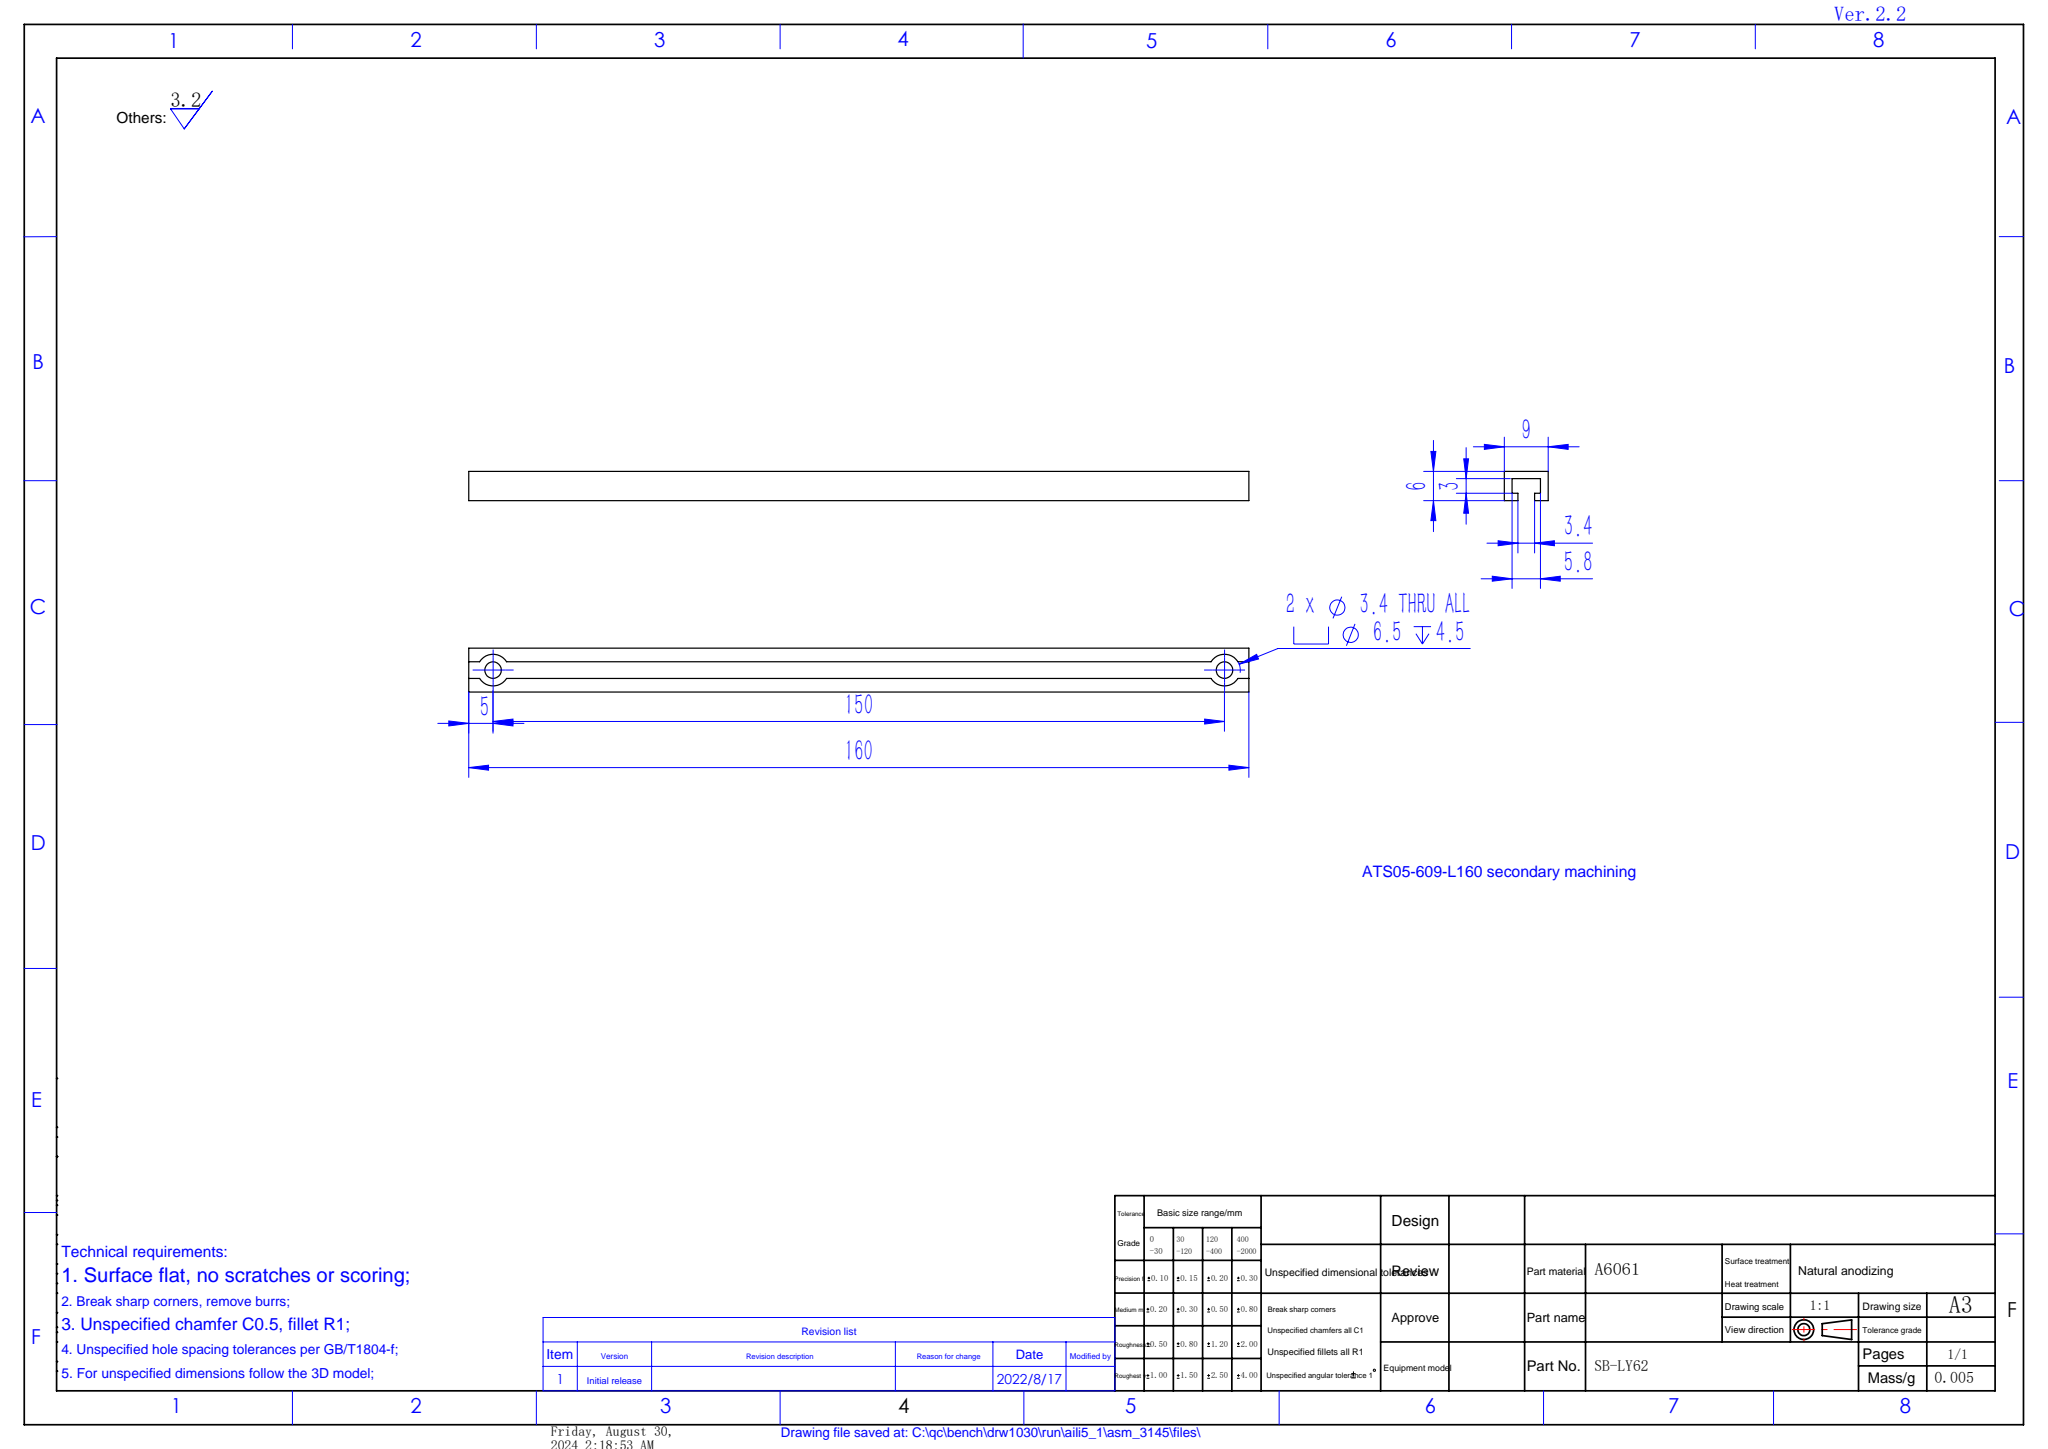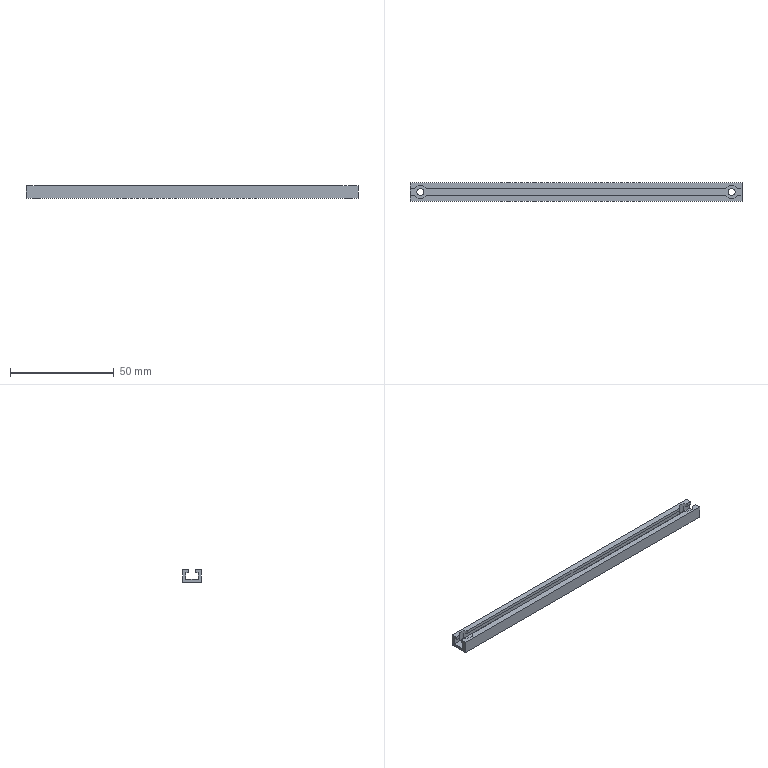Part | SolidWorks | features BaseBody 1, Cut 1, HoleWzd 1, ICE 1, MoveFace 1 | 1 solid | 34 faces | box 160 x 9 x 6 mm | volume 4968 mm3 | plane 26 | cylinder 8 | commonest cylinder face diameters 3.4 x4 6.5 x4